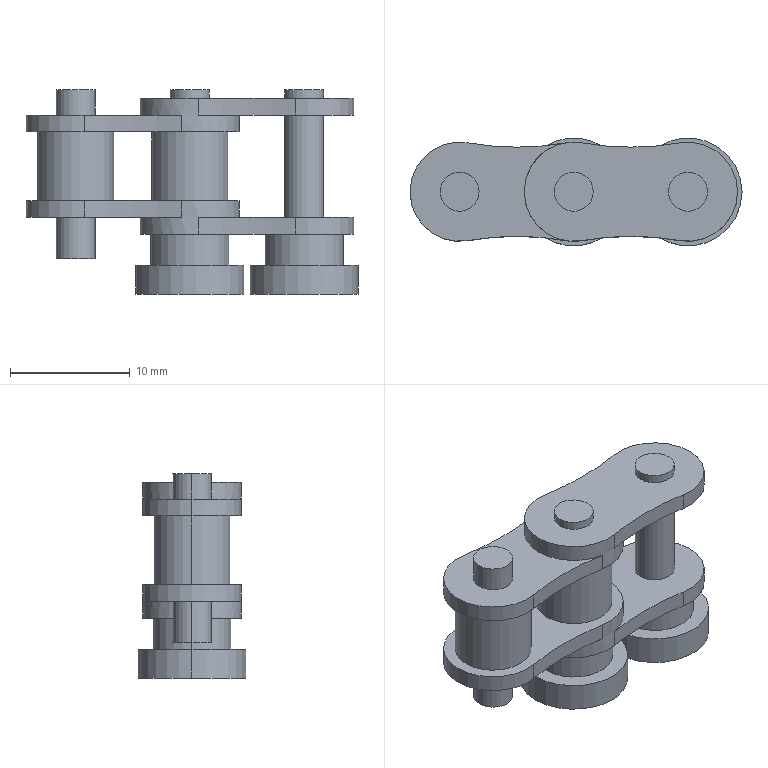Part | STEP file | 1 solid | 55 faces | box 27.685 x 9 x 17.043 mm | volume 1685 mm3 | cylinder 39 | plane 16 | commonest cylinder face diameters 3.25 x10 8.26 x9 47.072 x8 6.35 x4 6.5 x4 9 x4